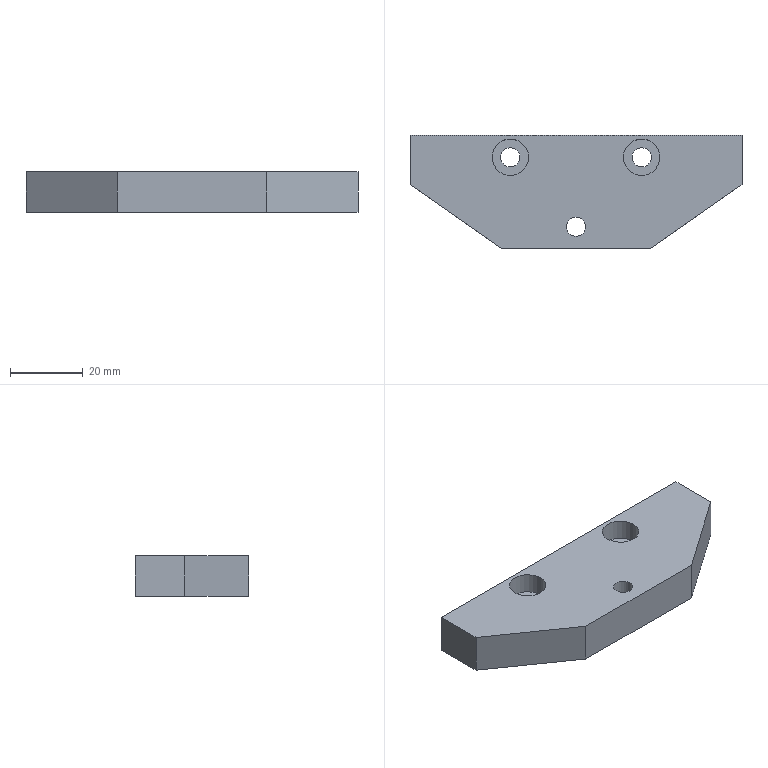Part | NX | 1 solid | 23 faces | box 91 x 31 x 11 mm | volume 24094 mm3 | plane 11 | cylinder 8 | cone 4 | commonest cylinder face diameters 5.3 x3 10 x3 4.2 x2
STEP:
#1=CARTESIAN_POINT('',(-15.35,9.5,0.));
#2=VERTEX_POINT('',#1);
#3=CARTESIAN_POINT('',(-18.,9.5,0.));
#4=DIRECTION('',(0.,0.,-1.));
#5=DIRECTION('',(1.,0.,0.));
#6=AXIS2_PLACEMENT_3D('',#3,#4,#5);
#7=CIRCLE('',#6,2.65);
#8=EDGE_CURVE('',#2,#2,#7,.T.);
#9=ORIENTED_EDGE('',*,*,#8,.T.);
#10=EDGE_LOOP('',(#9));
#11=FACE_BOUND('',#10,.T.);
#12=CARTESIAN_POINT('',(-15.35,9.5,5.3));
#13=VERTEX_POINT('',#12);
#14=CARTESIAN_POINT('',(-18.,9.5,5.3));
#15=DIRECTION('',(0.,0.,-1.));
#16=DIRECTION('',(1.,0.,0.));
#17=AXIS2_PLACEMENT_3D('',#14,#15,#16);
#18=CIRCLE('',#17,2.65);
#19=EDGE_CURVE('',#13,#13,#18,.T.);
#20=ORIENTED_EDGE('',*,*,#19,.F.);
#21=EDGE_LOOP('',(#20));
#22=FACE_BOUND('',#21,.T.);
#23=CARTESIAN_POINT('',(-18.,9.5,11.));
#24=DIRECTION('',(0.,0.,-1.));
#25=DIRECTION('',(1.,0.,0.));
#26=AXIS2_PLACEMENT_3D('',#23,#24,#25);
#27=CYLINDRICAL_SURFACE('',#26,2.65);
#28=ADVANCED_FACE('',(#11,#22),#27,.F.);
#29=CARTESIAN_POINT('',(-2.65,-9.5,11.));
#30=VERTEX_POINT('',#29);
#31=CARTESIAN_POINT('',(0.,-9.5,11.));
#32=DIRECTION('',(0.,0.,1.));
#33=DIRECTION('',(-1.,0.,0.));
#34=AXIS2_PLACEMENT_3D('',#31,#32,#33);
#35=CIRCLE('',#34,2.65);
#36=EDGE_CURVE('',#30,#30,#35,.T.);
#37=ORIENTED_EDGE('',*,*,#36,.F.);
#38=EDGE_LOOP('',(#37));
#39=FACE_BOUND('',#38,.T.);
#40=CARTESIAN_POINT('',(45.5,2.005,11.));
#41=VERTEX_POINT('',#40);
#42=CARTESIAN_POINT('',(45.5,15.5,11.));
#43=VERTEX_POINT('',#42);
#44=CARTESIAN_POINT('',(45.5,15.5,11.));
#45=DIRECTION('',(0.,1.,0.));
#46=VECTOR('',#45,1.);
#47=LINE('',#44,#46);
#48=EDGE_CURVE('',#41,#43,#47,.T.);
#49=ORIENTED_EDGE('',*,*,#48,.T.);
#50=CARTESIAN_POINT('',(-45.5,15.5,11.));
#51=VERTEX_POINT('',#50);
#52=CARTESIAN_POINT('',(-45.5,15.5,11.));
#53=DIRECTION('',(-1.,0.,0.));
#54=VECTOR('',#53,1.);
#55=LINE('',#52,#54);
#56=EDGE_CURVE('',#43,#51,#55,.T.);
#57=ORIENTED_EDGE('',*,*,#56,.T.);
#58=CARTESIAN_POINT('',(-45.5,2.005,11.));
#59=VERTEX_POINT('',#58);
#60=CARTESIAN_POINT('',(-45.5,2.005,11.));
#61=DIRECTION('',(0.,-1.,0.));
#62=VECTOR('',#61,1.);
#63=LINE('',#60,#62);
#64=EDGE_CURVE('',#51,#59,#63,.T.);
#65=ORIENTED_EDGE('',*,*,#64,.T.);
#66=CARTESIAN_POINT('',(-20.5,-15.5,11.));
#67=VERTEX_POINT('',#66);
#68=CARTESIAN_POINT('',(-20.5,-15.5,11.));
#69=DIRECTION('',(0.8192,-0.5736,0.));
#70=VECTOR('',#69,1.);
#71=LINE('',#68,#70);
#72=EDGE_CURVE('',#59,#67,#71,.T.);
#73=ORIENTED_EDGE('',*,*,#72,.T.);
#74=CARTESIAN_POINT('',(20.5,-15.5,11.));
#75=VERTEX_POINT('',#74);
#76=CARTESIAN_POINT('',(20.5,-15.5,11.));
#77=DIRECTION('',(1.,0.,0.));
#78=VECTOR('',#77,1.);
#79=LINE('',#76,#78);
#80=EDGE_CURVE('',#67,#75,#79,.T.);
#81=ORIENTED_EDGE('',*,*,#80,.T.);
#82=CARTESIAN_POINT('',(45.5,2.005,11.));
#83=DIRECTION('',(0.8192,0.5736,0.));
#84=VECTOR('',#83,1.);
#85=LINE('',#82,#84);
#86=EDGE_CURVE('',#75,#41,#85,.T.);
#87=ORIENTED_EDGE('',*,*,#86,.T.);
#88=EDGE_LOOP('',(#49,#57,#65,#73,#81,#87));
#89=FACE_BOUND('',#88,.T.);
#90=CARTESIAN_POINT('',(23.,9.5,11.));
#91=VERTEX_POINT('',#90);
#92=CARTESIAN_POINT('',(18.,9.5,11.));
#93=DIRECTION('',(0.,0.,-1.));
#94=DIRECTION('',(1.,0.,0.));
#95=AXIS2_PLACEMENT_3D('',#92,#93,#94);
#96=CIRCLE('',#95,5.);
#97=EDGE_CURVE('',#91,#91,#96,.T.);
#98=ORIENTED_EDGE('',*,*,#97,.T.);
#99=EDGE_LOOP('',(#98));
#100=FACE_BOUND('',#99,.T.);
#101=CARTESIAN_POINT('',(-13.,9.5,11.));
#102=VERTEX_POINT('',#101);
#103=CARTESIAN_POINT('',(-18.,9.5,11.));
#104=DIRECTION('',(0.,0.,1.));
#105=DIRECTION('',(1.,0.,0.));
#106=AXIS2_PLACEMENT_3D('',#103,#104,#105);
#107=CIRCLE('',#106,5.);
#108=EDGE_CURVE('',#102,#102,#107,.T.);
#109=ORIENTED_EDGE('',*,*,#108,.F.);
#110=EDGE_LOOP('',(#109));
#111=FACE_BOUND('',#110,.T.);
#112=CARTESIAN_POINT('',(-18.,9.5,11.));
#113=DIRECTION('',(0.,0.,-1.));
#114=DIRECTION('',(1.,0.,0.));
#115=AXIS2_PLACEMENT_3D('',#112,#113,#114);
#116=PLANE('',#115);
#117=ADVANCED_FACE('',(#39,#89,#100,#111),#116,.F.);
#118=CARTESIAN_POINT('',(45.5,15.5,0.));
#119=VERTEX_POINT('',#118);
#120=CARTESIAN_POINT('',(45.5,2.005,0.));
#121=VERTEX_POINT('',#120);
#122=CARTESIAN_POINT('',(45.5,15.5,0.));
#123=DIRECTION('',(0.,-1.,0.));
#124=VECTOR('',#123,1.);
#125=LINE('',#122,#124);
#126=EDGE_CURVE('',#119,#121,#125,.T.);
#127=ORIENTED_EDGE('',*,*,#126,.F.);
#128=CARTESIAN_POINT('',(45.5,15.5,11.));
#129=DIRECTION('',(0.,0.,-1.));
#130=VECTOR('',#129,1.);
#131=LINE('',#128,#130);
#132=EDGE_CURVE('',#43,#119,#131,.T.);
#133=ORIENTED_EDGE('',*,*,#132,.F.);
#134=ORIENTED_EDGE('',*,*,#48,.F.);
#135=CARTESIAN_POINT('',(45.5,2.005,11.));
#136=DIRECTION('',(0.,0.,-1.));
#137=VECTOR('',#136,1.);
#138=LINE('',#135,#137);
#139=EDGE_CURVE('',#41,#121,#138,.T.);
#140=ORIENTED_EDGE('',*,*,#139,.T.);
#141=EDGE_LOOP('',(#127,#133,#134,#140));
#142=FACE_OUTER_BOUND('',#141,.T.);
#143=CARTESIAN_POINT('',(45.5,15.5,11.));
#144=DIRECTION('',(1.,0.,0.));
#145=DIRECTION('',(0.,0.,1.));
#146=AXIS2_PLACEMENT_3D('',#143,#144,#145);
#147=PLANE('',#146);
#148=ADVANCED_FACE('',(#142),#147,.T.);
#149=CARTESIAN_POINT('',(20.5,-15.5,0.));
#150=VERTEX_POINT('',#149);
#151=CARTESIAN_POINT('',(45.5,2.005,0.));
#152=DIRECTION('',(-0.8192,-0.5736,0.));
#153=VECTOR('',#152,1.);
#154=LINE('',#151,#153);
#155=EDGE_CURVE('',#121,#150,#154,.T.);
#156=ORIENTED_EDGE('',*,*,#155,.F.);
#157=ORIENTED_EDGE('',*,*,#139,.F.);
#158=ORIENTED_EDGE('',*,*,#86,.F.);
#159=CARTESIAN_POINT('',(20.5,-15.5,11.));
#160=DIRECTION('',(0.,0.,-1.));
#161=VECTOR('',#160,1.);
#162=LINE('',#159,#161);
#163=EDGE_CURVE('',#75,#150,#162,.T.);
#164=ORIENTED_EDGE('',*,*,#163,.T.);
#165=EDGE_LOOP('',(#156,#157,#158,#164));
#166=FACE_OUTER_BOUND('',#165,.T.);
#167=CARTESIAN_POINT('',(45.5,2.005,11.));
#168=DIRECTION('',(0.5736,-0.8192,0.));
#169=DIRECTION('',(-0.8192,-0.5736,0.));
#170=AXIS2_PLACEMENT_3D('',#167,#168,#169);
#171=PLANE('',#170);
#172=ADVANCED_FACE('',(#166),#171,.T.);
#173=CARTESIAN_POINT('',(-20.5,-15.5,0.));
#174=VERTEX_POINT('',#173);
#175=CARTESIAN_POINT('',(20.5,-15.5,0.));
#176=DIRECTION('',(-1.,0.,0.));
#177=VECTOR('',#176,1.);
#178=LINE('',#175,#177);
#179=EDGE_CURVE('',#150,#174,#178,.T.);
#180=ORIENTED_EDGE('',*,*,#179,.F.);
#181=ORIENTED_EDGE('',*,*,#163,.F.);
#182=ORIENTED_EDGE('',*,*,#80,.F.);
#183=CARTESIAN_POINT('',(-20.5,-15.5,11.));
#184=DIRECTION('',(0.,0.,-1.));
#185=VECTOR('',#184,1.);
#186=LINE('',#183,#185);
#187=EDGE_CURVE('',#67,#174,#186,.T.);
#188=ORIENTED_EDGE('',*,*,#187,.T.);
#189=EDGE_LOOP('',(#180,#181,#182,#188));
#190=FACE_OUTER_BOUND('',#189,.T.);
#191=CARTESIAN_POINT('',(20.5,-15.5,11.));
#192=DIRECTION('',(0.,-1.,0.));
#193=DIRECTION('',(0.,0.,1.));
#194=AXIS2_PLACEMENT_3D('',#191,#192,#193);
#195=PLANE('',#194);
#196=ADVANCED_FACE('',(#190),#195,.T.);
#197=CARTESIAN_POINT('',(-45.5,2.005,0.));
#198=VERTEX_POINT('',#197);
#199=CARTESIAN_POINT('',(-20.5,-15.5,0.));
#200=DIRECTION('',(-0.8192,0.5736,0.));
#201=VECTOR('',#200,1.);
#202=LINE('',#199,#201);
#203=EDGE_CURVE('',#174,#198,#202,.T.);
#204=ORIENTED_EDGE('',*,*,#203,.F.);
#205=ORIENTED_EDGE('',*,*,#187,.F.);
#206=ORIENTED_EDGE('',*,*,#72,.F.);
#207=CARTESIAN_POINT('',(-45.5,2.005,11.));
#208=DIRECTION('',(0.,0.,-1.));
#209=VECTOR('',#208,1.);
#210=LINE('',#207,#209);
#211=EDGE_CURVE('',#59,#198,#210,.T.);
#212=ORIENTED_EDGE('',*,*,#211,.T.);
#213=EDGE_LOOP('',(#204,#205,#206,#212));
#214=FACE_OUTER_BOUND('',#213,.T.);
#215=CARTESIAN_POINT('',(-20.5,-15.5,11.));
#216=DIRECTION('',(-0.5736,-0.8192,0.));
#217=DIRECTION('',(-0.8192,0.5736,0.));
#218=AXIS2_PLACEMENT_3D('',#215,#216,#217);
#219=PLANE('',#218);
#220=ADVANCED_FACE('',(#214),#219,.T.);
#221=CARTESIAN_POINT('',(-45.5,15.5,0.));
#222=VERTEX_POINT('',#221);
#223=CARTESIAN_POINT('',(-45.5,2.005,0.));
#224=DIRECTION('',(0.,1.,0.));
#225=VECTOR('',#224,1.);
#226=LINE('',#223,#225);
#227=EDGE_CURVE('',#198,#222,#226,.T.);
#228=ORIENTED_EDGE('',*,*,#227,.F.);
#229=ORIENTED_EDGE('',*,*,#211,.F.);
#230=ORIENTED_EDGE('',*,*,#64,.F.);
#231=CARTESIAN_POINT('',(-45.5,15.5,11.));
#232=DIRECTION('',(0.,0.,-1.));
#233=VECTOR('',#232,1.);
#234=LINE('',#231,#233);
#235=EDGE_CURVE('',#51,#222,#234,.T.);
#236=ORIENTED_EDGE('',*,*,#235,.T.);
#237=EDGE_LOOP('',(#228,#229,#230,#236));
#238=FACE_OUTER_BOUND('',#237,.T.);
#239=CARTESIAN_POINT('',(-45.5,2.005,11.));
#240=DIRECTION('',(-1.,0.,0.));
#241=DIRECTION('',(0.,0.,-1.));
#242=AXIS2_PLACEMENT_3D('',#239,#240,#241);
#243=PLANE('',#242);
#244=ADVANCED_FACE('',(#238),#243,.T.);
#245=CARTESIAN_POINT('',(2.65,-9.5,5.7));
#246=VERTEX_POINT('',#245);
#247=CARTESIAN_POINT('',(0.,-9.5,5.7));
#248=DIRECTION('',(0.,0.,-1.));
#249=DIRECTION('',(1.,0.,0.));
#250=AXIS2_PLACEMENT_3D('',#247,#248,#249);
#251=CIRCLE('',#250,2.65);
#252=EDGE_CURVE('',#246,#246,#251,.T.);
#253=ORIENTED_EDGE('',*,*,#252,.T.);
#254=EDGE_LOOP('',(#253));
#255=FACE_BOUND('',#254,.T.);
#256=ORIENTED_EDGE('',*,*,#36,.T.);
#257=EDGE_LOOP('',(#256));
#258=FACE_BOUND('',#257,.T.);
#259=CARTESIAN_POINT('',(0.,-9.5,11.));
#260=DIRECTION('',(0.,0.,-1.));
#261=DIRECTION('',(1.,0.,0.));
#262=AXIS2_PLACEMENT_3D('',#259,#260,#261);
#263=CYLINDRICAL_SURFACE('',#262,2.65);
#264=ADVANCED_FACE('',(#255,#258),#263,.F.);
#265=CARTESIAN_POINT('',(40.5,15.5,8.));
#266=VERTEX_POINT('',#265);
#267=CARTESIAN_POINT('',(40.5,15.5,5.5));
#268=DIRECTION('',(0.,-1.,0.));
#269=DIRECTION('',(0.,0.,1.));
#270=AXIS2_PLACEMENT_3D('',#267,#268,#269);
#271=CIRCLE('',#270,2.5);
#272=EDGE_CURVE('',#266,#266,#271,.T.);
#273=ORIENTED_EDGE('',*,*,#272,.T.);
#274=EDGE_LOOP('',(#273));
#275=FACE_BOUND('',#274,.T.);
#276=CARTESIAN_POINT('',(-40.5,15.5,8.));
#277=VERTEX_POINT('',#276);
#278=CARTESIAN_POINT('',(-40.5,15.5,5.5));
#279=DIRECTION('',(0.,-1.,0.));
#280=DIRECTION('',(0.,0.,1.));
#281=AXIS2_PLACEMENT_3D('',#278,#279,#280);
#282=CIRCLE('',#281,2.5);
#283=EDGE_CURVE('',#277,#277,#282,.T.);
#284=ORIENTED_EDGE('',*,*,#283,.T.);
#285=EDGE_LOOP('',(#284));
#286=FACE_BOUND('',#285,.T.);
#287=CARTESIAN_POINT('',(-45.5,15.5,0.));
#288=DIRECTION('',(1.,0.,0.));
#289=VECTOR('',#288,1.);
#290=LINE('',#287,#289);
#291=EDGE_CURVE('',#222,#119,#290,.T.);
#292=ORIENTED_EDGE('',*,*,#291,.F.);
#293=ORIENTED_EDGE('',*,*,#235,.F.);
#294=ORIENTED_EDGE('',*,*,#56,.F.);
#295=ORIENTED_EDGE('',*,*,#132,.T.);
#296=EDGE_LOOP('',(#292,#293,#294,#295));
#297=FACE_BOUND('',#296,.T.);
#298=CARTESIAN_POINT('',(-45.5,15.5,11.));
#299=DIRECTION('',(0.,1.,0.));
#300=DIRECTION('',(0.,0.,-1.));
#301=AXIS2_PLACEMENT_3D('',#298,#299,#300);
#302=PLANE('',#301);
#303=ADVANCED_FACE('',(#275,#286,#297),#302,.T.);
#304=CARTESIAN_POINT('',(15.35,9.5,5.3));
#305=VERTEX_POINT('',#304);
#306=CARTESIAN_POINT('',(18.,9.5,5.3));
#307=DIRECTION('',(0.,0.,1.));
#308=DIRECTION('',(-1.,0.,0.));
#309=AXIS2_PLACEMENT_3D('',#306,#307,#308);
#310=CIRCLE('',#309,2.65);
#311=EDGE_CURVE('',#305,#305,#310,.T.);
#312=ORIENTED_EDGE('',*,*,#311,.T.);
#313=EDGE_LOOP('',(#312));
#314=FACE_BOUND('',#313,.T.);
#315=CARTESIAN_POINT('',(20.65,9.5,0.));
#316=VERTEX_POINT('',#315);
#317=CARTESIAN_POINT('',(18.,9.5,0.));
#318=DIRECTION('',(0.,0.,-1.));
#319=DIRECTION('',(1.,0.,0.));
#320=AXIS2_PLACEMENT_3D('',#317,#318,#319);
#321=CIRCLE('',#320,2.65);
#322=EDGE_CURVE('',#316,#316,#321,.T.);
#323=ORIENTED_EDGE('',*,*,#322,.T.);
#324=EDGE_LOOP('',(#323));
#325=FACE_BOUND('',#324,.T.);
#326=CARTESIAN_POINT('',(18.,9.5,11.));
#327=DIRECTION('',(0.,0.,-1.));
#328=DIRECTION('',(1.,0.,0.));
#329=AXIS2_PLACEMENT_3D('',#326,#327,#328);
#330=CYLINDRICAL_SURFACE('',#329,2.65);
#331=ADVANCED_FACE('',(#314,#325),#330,.F.);
#332=CARTESIAN_POINT('',(-5.,-9.5,0.));
#333=VERTEX_POINT('',#332);
#334=CARTESIAN_POINT('',(0.,-9.5,0.));
#335=DIRECTION('',(0.,0.,1.));
#336=DIRECTION('',(-1.,0.,0.));
#337=AXIS2_PLACEMENT_3D('',#334,#335,#336);
#338=CIRCLE('',#337,5.);
#339=EDGE_CURVE('',#333,#333,#338,.T.);
#340=ORIENTED_EDGE('',*,*,#339,.T.);
#341=EDGE_LOOP('',(#340));
#342=FACE_BOUND('',#341,.T.);
#343=ORIENTED_EDGE('',*,*,#126,.T.);
#344=ORIENTED_EDGE('',*,*,#155,.T.);
#345=ORIENTED_EDGE('',*,*,#179,.T.);
#346=ORIENTED_EDGE('',*,*,#203,.T.);
#347=ORIENTED_EDGE('',*,*,#227,.T.);
#348=ORIENTED_EDGE('',*,*,#291,.T.);
#349=EDGE_LOOP('',(#343,#344,#345,#346,#347,#348));
#350=FACE_BOUND('',#349,.T.);
#351=ORIENTED_EDGE('',*,*,#8,.F.);
#352=EDGE_LOOP('',(#351));
#353=FACE_BOUND('',#352,.T.);
#354=ORIENTED_EDGE('',*,*,#322,.F.);
#355=EDGE_LOOP('',(#354));
#356=FACE_BOUND('',#355,.T.);
#357=CARTESIAN_POINT('',(-18.,9.5,0.));
#358=DIRECTION('',(0.,0.,-1.));
#359=DIRECTION('',(1.,0.,0.));
#360=AXIS2_PLACEMENT_3D('',#357,#358,#359);
#361=PLANE('',#360);
#362=ADVANCED_FACE('',(#342,#350,#353,#356),#361,.T.);
#363=CARTESIAN_POINT('',(23.,9.5,5.3));
#364=VERTEX_POINT('',#363);
#365=CARTESIAN_POINT('',(18.,9.5,5.3));
#366=DIRECTION('',(0.,0.,1.));
#367=DIRECTION('',(1.,0.,0.));
#368=AXIS2_PLACEMENT_3D('',#365,#366,#367);
#369=CIRCLE('',#368,5.);
#370=EDGE_CURVE('',#364,#364,#369,.T.);
#371=ORIENTED_EDGE('',*,*,#370,.T.);
#372=EDGE_LOOP('',(#371));
#373=FACE_BOUND('',#372,.T.);
#374=ORIENTED_EDGE('',*,*,#311,.F.);
#375=EDGE_LOOP('',(#374));
#376=FACE_BOUND('',#375,.T.);
#377=CARTESIAN_POINT('',(18.,9.5,5.3));
#378=DIRECTION('',(0.,0.,-1.));
#379=DIRECTION('',(1.,0.,0.));
#380=AXIS2_PLACEMENT_3D('',#377,#378,#379);
#381=PLANE('',#380);
#382=ADVANCED_FACE('',(#373,#376),#381,.F.);
#383=ORIENTED_EDGE('',*,*,#370,.F.);
#384=EDGE_LOOP('',(#383));
#385=FACE_BOUND('',#384,.T.);
#386=ORIENTED_EDGE('',*,*,#97,.F.);
#387=EDGE_LOOP('',(#386));
#388=FACE_BOUND('',#387,.T.);
#389=CARTESIAN_POINT('',(18.,9.5,11.));
#390=DIRECTION('',(0.,0.,-1.));
#391=DIRECTION('',(1.,0.,0.));
#392=AXIS2_PLACEMENT_3D('',#389,#390,#391);
#393=CYLINDRICAL_SURFACE('',#392,5.);
#394=ADVANCED_FACE('',(#385,#388),#393,.F.);
#395=CARTESIAN_POINT('',(-13.,9.5,5.3));
#396=VERTEX_POINT('',#395);
#397=CARTESIAN_POINT('',(-18.,9.5,5.3));
#398=DIRECTION('',(0.,0.,-1.));
#399=DIRECTION('',(1.,0.,0.));
#400=AXIS2_PLACEMENT_3D('',#397,#398,#399);
#401=CIRCLE('',#400,5.);
#402=EDGE_CURVE('',#396,#396,#401,.T.);
#403=ORIENTED_EDGE('',*,*,#402,.F.);
#404=EDGE_LOOP('',(#403));
#405=FACE_BOUND('',#404,.T.);
#406=ORIENTED_EDGE('',*,*,#19,.T.);
#407=EDGE_LOOP('',(#406));
#408=FACE_BOUND('',#407,.T.);
#409=CARTESIAN_POINT('',(-18.,9.5,5.3));
#410=DIRECTION('',(0.,0.,1.));
#411=DIRECTION('',(-1.,0.,0.));
#412=AXIS2_PLACEMENT_3D('',#409,#410,#411);
#413=PLANE('',#412);
#414=ADVANCED_FACE('',(#405,#408),#413,.T.);
#415=ORIENTED_EDGE('',*,*,#402,.T.);
#416=EDGE_LOOP('',(#415));
#417=FACE_BOUND('',#416,.T.);
#418=ORIENTED_EDGE('',*,*,#108,.T.);
#419=EDGE_LOOP('',(#418));
#420=FACE_BOUND('',#419,.T.);
#421=CARTESIAN_POINT('',(-18.,9.5,11.));
#422=DIRECTION('',(0.,0.,-1.));
#423=DIRECTION('',(1.,0.,0.));
#424=AXIS2_PLACEMENT_3D('',#421,#422,#423);
#425=CYLINDRICAL_SURFACE('',#424,5.);
#426=ADVANCED_FACE('',(#417,#420),#425,.F.);
#427=CARTESIAN_POINT('',(-5.,-9.5,5.7));
#428=VERTEX_POINT('',#427);
#429=CARTESIAN_POINT('',(0.,-9.5,5.7));
#430=DIRECTION('',(0.,0.,-1.));
#431=DIRECTION('',(-1.,0.,0.));
#432=AXIS2_PLACEMENT_3D('',#429,#430,#431);
#433=CIRCLE('',#432,5.);
#434=EDGE_CURVE('',#428,#428,#433,.T.);
#435=ORIENTED_EDGE('',*,*,#434,.T.);
#436=EDGE_LOOP('',(#435));
#437=FACE_BOUND('',#436,.T.);
#438=ORIENTED_EDGE('',*,*,#252,.F.);
#439=EDGE_LOOP('',(#438));
#440=FACE_BOUND('',#439,.T.);
#441=CARTESIAN_POINT('',(0.,-9.5,5.7));
#442=DIRECTION('',(0.,0.,1.));
#443=DIRECTION('',(-1.,0.,0.));
#444=AXIS2_PLACEMENT_3D('',#441,#442,#443);
#445=PLANE('',#444);
#446=ADVANCED_FACE('',(#437,#440),#445,.F.);
#447=ORIENTED_EDGE('',*,*,#339,.F.);
#448=EDGE_LOOP('',(#447));
#449=FACE_BOUND('',#448,.T.);
#450=ORIENTED_EDGE('',*,*,#434,.F.);
#451=EDGE_LOOP('',(#450));
#452=FACE_BOUND('',#451,.T.);
#453=CARTESIAN_POINT('',(0.,-9.5,5.7));
#454=DIRECTION('',(0.,0.,-1.));
#455=DIRECTION('',(1.,0.,0.));
#456=AXIS2_PLACEMENT_3D('',#453,#454,#455);
#457=CYLINDRICAL_SURFACE('',#456,5.);
#458=ADVANCED_FACE('',(#449,#452),#457,.F.);
#459=CARTESIAN_POINT('',(-40.5,0.5,3.4));
#460=VERTEX_POINT('',#459);
#461=CARTESIAN_POINT('',(-40.5,0.5,5.5));
#462=DIRECTION('',(0.,1.,0.));
#463=DIRECTION('',(0.,0.,-1.));
#464=AXIS2_PLACEMENT_3D('',#461,#462,#463);
#465=CIRCLE('',#464,2.1);
#466=EDGE_CURVE('',#460,#460,#465,.T.);
#467=ORIENTED_EDGE('',*,*,#466,.T.);
#468=EDGE_LOOP('',(#467));
#469=FACE_BOUND('',#468,.T.);
#470=CARTESIAN_POINT('',(-40.5,-0.7618,5.5));
#471=VERTEX_POINT('',#470);
#472=VERTEX_LOOP('',#471);
#473=FACE_BOUND('',#472,.T.);
#474=CARTESIAN_POINT('',(-40.5,0.5,5.5));
#475=DIRECTION('',(0.,1.,0.));
#476=DIRECTION('',(0.,0.,-1.));
#477=AXIS2_PLACEMENT_3D('',#474,#475,#476);
#478=CONICAL_SURFACE('',#477,2.1,59.);
#479=ADVANCED_FACE('',(#469,#473),#478,.F.);
#480=CARTESIAN_POINT('',(-40.5,15.1,7.6));
#481=VERTEX_POINT('',#480);
#482=CARTESIAN_POINT('',(-40.5,15.1,5.5));
#483=DIRECTION('',(0.,1.,0.));
#484=DIRECTION('',(0.,0.,1.));
#485=AXIS2_PLACEMENT_3D('',#482,#483,#484);
#486=CIRCLE('',#485,2.1);
#487=EDGE_CURVE('',#481,#481,#486,.T.);
#488=ORIENTED_EDGE('',*,*,#487,.T.);
#489=EDGE_LOOP('',(#488));
#490=FACE_BOUND('',#489,.T.);
#491=ORIENTED_EDGE('',*,*,#466,.F.);
#492=EDGE_LOOP('',(#491));
#493=FACE_BOUND('',#492,.T.);
#494=CARTESIAN_POINT('',(-40.5,15.5,5.5));
#495=DIRECTION('',(0.,-1.,0.));
#496=DIRECTION('',(0.,0.,1.));
#497=AXIS2_PLACEMENT_3D('',#494,#495,#496);
#498=CYLINDRICAL_SURFACE('',#497,2.1);
#499=ADVANCED_FACE('',(#490,#493),#498,.F.);
#500=ORIENTED_EDGE('',*,*,#487,.F.);
#501=EDGE_LOOP('',(#500));
#502=FACE_BOUND('',#501,.T.);
#503=ORIENTED_EDGE('',*,*,#283,.F.);
#504=EDGE_LOOP('',(#503));
#505=FACE_BOUND('',#504,.T.);
#506=CARTESIAN_POINT('',(-40.5,15.5,5.5));
#507=DIRECTION('',(0.,1.,0.));
#508=DIRECTION('',(0.,0.,-1.));
#509=AXIS2_PLACEMENT_3D('',#506,#507,#508);
#510=CONICAL_SURFACE('',#509,2.5,45.);
#511=ADVANCED_FACE('',(#502,#505),#510,.F.);
#512=CARTESIAN_POINT('',(40.5,0.5,3.4));
#513=VERTEX_POINT('',#512);
#514=CARTESIAN_POINT('',(40.5,0.5,5.5));
#515=DIRECTION('',(0.,1.,0.));
#516=DIRECTION('',(0.,0.,-1.));
#517=AXIS2_PLACEMENT_3D('',#514,#515,#516);
#518=CIRCLE('',#517,2.1);
#519=EDGE_CURVE('',#513,#513,#518,.T.);
#520=ORIENTED_EDGE('',*,*,#519,.T.);
#521=EDGE_LOOP('',(#520));
#522=FACE_BOUND('',#521,.T.);
#523=CARTESIAN_POINT('',(40.5,-0.7618,5.5));
#524=VERTEX_POINT('',#523);
#525=VERTEX_LOOP('',#524);
#526=FACE_BOUND('',#525,.T.);
#527=CARTESIAN_POINT('',(40.5,0.5,5.5));
#528=DIRECTION('',(0.,1.,0.));
#529=DIRECTION('',(0.,0.,-1.));
#530=AXIS2_PLACEMENT_3D('',#527,#528,#529);
#531=CONICAL_SURFACE('',#530,2.1,59.);
#532=ADVANCED_FACE('',(#522,#526),#531,.F.);
#533=CARTESIAN_POINT('',(40.5,15.1,7.6));
#534=VERTEX_POINT('',#533);
#535=CARTESIAN_POINT('',(40.5,15.1,5.5));
#536=DIRECTION('',(0.,1.,0.));
#537=DIRECTION('',(0.,0.,1.));
#538=AXIS2_PLACEMENT_3D('',#535,#536,#537);
#539=CIRCLE('',#538,2.1);
#540=EDGE_CURVE('',#534,#534,#539,.T.);
#541=ORIENTED_EDGE('',*,*,#540,.T.);
#542=EDGE_LOOP('',(#541));
#543=FACE_BOUND('',#542,.T.);
#544=ORIENTED_EDGE('',*,*,#519,.F.);
#545=EDGE_LOOP('',(#544));
#546=FACE_BOUND('',#545,.T.);
#547=CARTESIAN_POINT('',(40.5,15.5,5.5));
#548=DIRECTION('',(0.,-1.,0.));
#549=DIRECTION('',(0.,0.,1.));
#550=AXIS2_PLACEMENT_3D('',#547,#548,#549);
#551=CYLINDRICAL_SURFACE('',#550,2.1);
#552=ADVANCED_FACE('',(#543,#546),#551,.F.);
#553=ORIENTED_EDGE('',*,*,#540,.F.);
#554=EDGE_LOOP('',(#553));
#555=FACE_BOUND('',#554,.T.);
#556=ORIENTED_EDGE('',*,*,#272,.F.);
#557=EDGE_LOOP('',(#556));
#558=FACE_BOUND('',#557,.T.);
#559=CARTESIAN_POINT('',(40.5,15.5,5.5));
#560=DIRECTION('',(0.,1.,0.));
#561=DIRECTION('',(0.,0.,-1.));
#562=AXIS2_PLACEMENT_3D('',#559,#560,#561);
#563=CONICAL_SURFACE('',#562,2.5,45.);
#564=ADVANCED_FACE('',(#555,#558),#563,.F.);
#565=CLOSED_SHELL('',(#28,#117,#148,#172,#196,#220,#244,#264,#303,#331,#362,#382,#394,#414,#426,#446,#458,#479,#499,#511,#532,#552,#564));
#566=MANIFOLD_SOLID_BREP('',#565);
#567=(LENGTH_UNIT()NAMED_UNIT(*)SI_UNIT(.MILLI.,.METRE.));
#568=UNCERTAINTY_MEASURE_WITH_UNIT(LENGTH_MEASURE(0.00002),#567,'','');
#569=(NAMED_UNIT(*)PLANE_ANGLE_UNIT()SI_UNIT($,.RADIAN.));
#570=PLANE_ANGLE_MEASURE_WITH_UNIT(PLANE_ANGLE_MEASURE(0.01745),#569);
#571=DIMENSIONAL_EXPONENTS(0.,0.,0.,0.,0.,0.,0.);
#572=(CONVERSION_BASED_UNIT('DEGREE',#570)NAMED_UNIT(#571)PLANE_ANGLE_UNIT());
#573=(NAMED_UNIT(*)SI_UNIT($,.STERADIAN.)SOLID_ANGLE_UNIT());
#574=(GEOMETRIC_REPRESENTATION_CONTEXT(3)GLOBAL_UNCERTAINTY_ASSIGNED_CONTEXT((#568))GLOBAL_UNIT_ASSIGNED_CONTEXT((#567,#572,#573))REPRESENTATION_CONTEXT('',''));
#575=ADVANCED_BREP_SHAPE_REPRESENTATION('',(#566),#574);